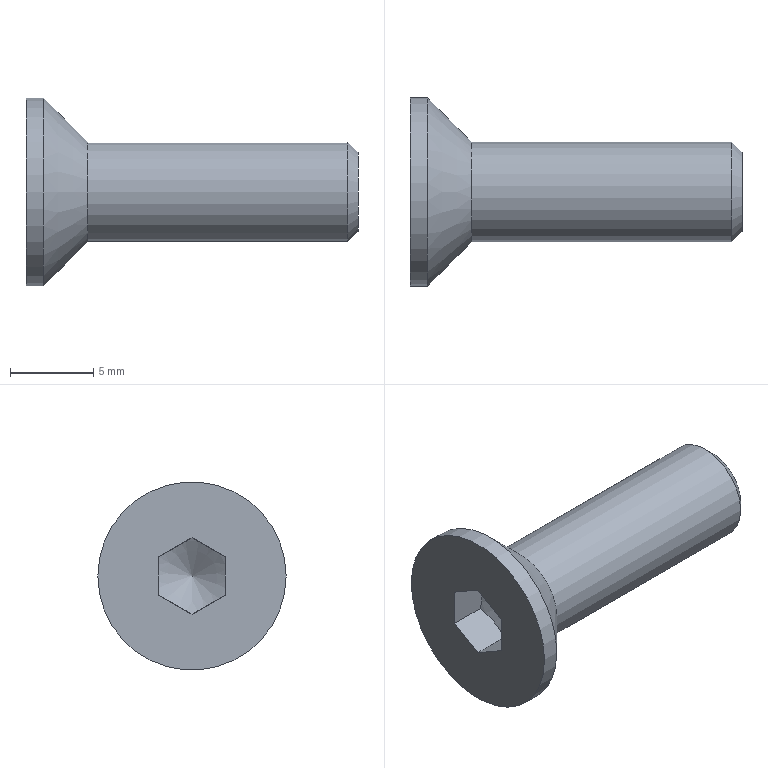Part | STEP file | DIN 7991 - M6  x  20 | 1 solid | 13 faces | box 20 x 11.34 x 11.34 mm | volume 687.937 mm3 | plane 8 | cone 3 | cylinder 2 | commonest cylinder face diameters 6 x1 11.34 x1
STEP:
#1=CARTESIAN_POINT('',(0.,0.,0.));
#2=DIRECTION('',(0.,0.,1.));
#3=DIRECTION('',(1.,0.,0.));
#4=AXIS2_PLACEMENT_3D('',#1,#2,#3);
#5=CARTESIAN_POINT('',(19.387,3.,0.));
#6=VERTEX_POINT('',#5);
#7=CARTESIAN_POINT('',(19.387,0.,0.));
#8=DIRECTION('',(1.,0.,0.));
#9=DIRECTION('',(0.,-1.,0.));
#10=AXIS2_PLACEMENT_3D('',#7,#8,#9);
#11=CIRCLE('',#10,3.);
#12=CARTESIAN_POINT('',(19.693,0.,0.));
#13=DIRECTION('',(-1.,0.,0.));
#14=DIRECTION('',(0.,-1.,0.));
#15=AXIS2_PLACEMENT_3D('',#12,#13,#14);
#16=CONICAL_SURFACE('',#15,2.693,0.7854);
#17=CARTESIAN_POINT('',(12.566,0.3067));
#18=DIRECTION('',(-1.,0.));
#19=VECTOR('',#18,1.);
#20=LINE('',#17,#19);
#21=(GEOMETRIC_REPRESENTATION_CONTEXT(2)PARAMETRIC_REPRESENTATION_CONTEXT()REPRESENTATION_CONTEXT('',''));
#22=DEFINITIONAL_REPRESENTATION('',(#20),#21);
#23=PCURVE('',#16,#22);
#24=CARTESIAN_POINT('',(13.5,0.,0.));
#25=DIRECTION('',(1.,0.,0.));
#26=DIRECTION('',(0.,1.,0.));
#27=AXIS2_PLACEMENT_3D('',#24,#25,#26);
#28=CYLINDRICAL_SURFACE('',#27,3.);
#29=CARTESIAN_POINT('',(-3.142,5.887));
#30=DIRECTION('',(1.,0.));
#31=VECTOR('',#30,1.);
#32=LINE('',#29,#31);
#33=(GEOMETRIC_REPRESENTATION_CONTEXT(2)PARAMETRIC_REPRESENTATION_CONTEXT()REPRESENTATION_CONTEXT('',''));
#34=DEFINITIONAL_REPRESENTATION('',(#32),#33);
#35=PCURVE('',#28,#34);
#36=SURFACE_CURVE('',#11,(#23,#35),.PCURVE_S1.);
#37=EDGE_CURVE('',#6,#6,#36,.T.);
#38=ORIENTED_EDGE('',*,*,#37,.T.);
#39=CARTESIAN_POINT('',(20.,2.387,0.));
#40=VERTEX_POINT('',#39);
#41=CARTESIAN_POINT('',(20.,2.387,0.));
#42=CARTESIAN_POINT('',(19.387,3.,0.));
#43=B_SPLINE_CURVE_WITH_KNOTS('',1,(#41,#42),.UNSPECIFIED.,.F.,.F.,(2,2),(-0.4338,0.4338),.PIECEWISE_BEZIER_KNOTS.);
#44=CARTESIAN_POINT('',(3.142,0.));
#45=DIRECTION('',(0.,1.));
#46=VECTOR('',#45,1.);
#47=LINE('',#44,#46);
#48=(GEOMETRIC_REPRESENTATION_CONTEXT(2)PARAMETRIC_REPRESENTATION_CONTEXT()REPRESENTATION_CONTEXT('',''));
#49=DEFINITIONAL_REPRESENTATION('',(#47),#48);
#50=PCURVE('',#16,#49);
#51=CARTESIAN_POINT('',(9.425,0.));
#52=DIRECTION('',(0.,1.));
#53=VECTOR('',#52,1.);
#54=LINE('',#51,#53);
#55=(GEOMETRIC_REPRESENTATION_CONTEXT(2)PARAMETRIC_REPRESENTATION_CONTEXT()REPRESENTATION_CONTEXT('',''));
#56=DEFINITIONAL_REPRESENTATION('',(#54),#55);
#57=PCURVE('',#16,#56);
#58=SEAM_CURVE('',#43,(#50,#57),.PCURVE_S1.);
#59=EDGE_CURVE('',#40,#6,#58,.T.);
#60=ORIENTED_EDGE('',*,*,#59,.F.);
#61=CARTESIAN_POINT('',(20.,0.,0.));
#62=DIRECTION('',(-1.,0.,0.));
#63=DIRECTION('',(0.,-1.,0.));
#64=AXIS2_PLACEMENT_3D('',#61,#62,#63);
#65=CIRCLE('',#64,2.387);
#66=CARTESIAN_POINT('',(0.,-0.3067));
#67=DIRECTION('',(1.,0.));
#68=VECTOR('',#67,1.);
#69=LINE('',#66,#68);
#70=(GEOMETRIC_REPRESENTATION_CONTEXT(2)PARAMETRIC_REPRESENTATION_CONTEXT()REPRESENTATION_CONTEXT('',''));
#71=DEFINITIONAL_REPRESENTATION('',(#69),#70);
#72=PCURVE('',#16,#71);
#73=CARTESIAN_POINT('',(20.,1.5,0.));
#74=DIRECTION('',(1.,0.,0.));
#75=DIRECTION('',(0.,0.,-1.));
#76=AXIS2_PLACEMENT_3D('',#73,#74,#75);
#77=PLANE('',#76);
#78=CARTESIAN_POINT('',(0.,-3.887));
#79=CARTESIAN_POINT('',(-4.134,-3.887));
#80=CARTESIAN_POINT('',(-2.067,-0.3067));
#81=CARTESIAN_POINT('',(0.,3.273));
#82=CARTESIAN_POINT('',(2.067,-0.3067));
#83=CARTESIAN_POINT('',(4.134,-3.887));
#84=CARTESIAN_POINT('',(0.,-3.887));
#85=(BOUNDED_CURVE()B_SPLINE_CURVE(2,(#78,#79,#80,#81,#82,#83,#84),.UNSPECIFIED.,.T.,.F.)B_SPLINE_CURVE_WITH_KNOTS((1,2,2,2,2,1),(-2.094,0.,2.094,4.189,6.283,8.378),.UNSPECIFIED.)CURVE()GEOMETRIC_REPRESENTATION_ITEM()RATIONAL_B_SPLINE_CURVE((1.,0.5,1.,0.5,1.,0.5,1.))REPRESENTATION_ITEM(''));
#86=(GEOMETRIC_REPRESENTATION_CONTEXT(2)PARAMETRIC_REPRESENTATION_CONTEXT()REPRESENTATION_CONTEXT('',''));
#87=DEFINITIONAL_REPRESENTATION('',(#85),#86);
#88=PCURVE('',#77,#87);
#89=SURFACE_CURVE('',#65,(#72,#88),.PCURVE_S1.);
#90=EDGE_CURVE('',#40,#40,#89,.T.);
#91=ORIENTED_EDGE('',*,*,#90,.T.);
#92=ORIENTED_EDGE('',*,*,#59,.T.);
#93=EDGE_LOOP('',(#38,#60,#91,#92));
#94=FACE_BOUND('',#93,.T.);
#95=ADVANCED_FACE('',(#94),#16,.T.);
#96=CARTESIAN_POINT('',(3.72,3.,0.));
#97=VERTEX_POINT('',#96);
#98=CARTESIAN_POINT('',(3.72,0.,0.));
#99=DIRECTION('',(1.,0.,0.));
#100=DIRECTION('',(0.,1.,0.));
#101=AXIS2_PLACEMENT_3D('',#98,#99,#100);
#102=CIRCLE('',#101,3.);
#103=CARTESIAN_POINT('',(0.,-9.78));
#104=DIRECTION('',(1.,0.));
#105=VECTOR('',#104,1.);
#106=LINE('',#103,#105);
#107=(GEOMETRIC_REPRESENTATION_CONTEXT(2)PARAMETRIC_REPRESENTATION_CONTEXT()REPRESENTATION_CONTEXT('',''));
#108=DEFINITIONAL_REPRESENTATION('',(#106),#107);
#109=PCURVE('',#28,#108);
#110=CARTESIAN_POINT('',(2.385,0.,0.));
#111=DIRECTION('',(-1.,0.,0.));
#112=DIRECTION('',(0.,1.,0.));
#113=AXIS2_PLACEMENT_3D('',#110,#111,#112);
#114=CONICAL_SURFACE('',#113,4.335,0.7854);
#115=CARTESIAN_POINT('',(6.283,-1.335));
#116=DIRECTION('',(-1.,0.));
#117=VECTOR('',#116,1.);
#118=LINE('',#115,#117);
#119=(GEOMETRIC_REPRESENTATION_CONTEXT(2)PARAMETRIC_REPRESENTATION_CONTEXT()REPRESENTATION_CONTEXT('',''));
#120=DEFINITIONAL_REPRESENTATION('',(#118),#119);
#121=PCURVE('',#114,#120);
#122=SURFACE_CURVE('',#102,(#109,#121),.PCURVE_S1.);
#123=EDGE_CURVE('',#97,#97,#122,.T.);
#124=ORIENTED_EDGE('',*,*,#123,.T.);
#125=CARTESIAN_POINT('',(3.72,3.,0.));
#126=CARTESIAN_POINT('',(19.387,3.,0.));
#127=B_SPLINE_CURVE_WITH_KNOTS('',1,(#125,#126),.UNSPECIFIED.,.F.,.F.,(2,2),(-9.78,5.887),.PIECEWISE_BEZIER_KNOTS.);
#128=CARTESIAN_POINT('',(6.283,0.));
#129=DIRECTION('',(0.,1.));
#130=VECTOR('',#129,1.);
#131=LINE('',#128,#130);
#132=(GEOMETRIC_REPRESENTATION_CONTEXT(2)PARAMETRIC_REPRESENTATION_CONTEXT()REPRESENTATION_CONTEXT('',''));
#133=DEFINITIONAL_REPRESENTATION('',(#131),#132);
#134=PCURVE('',#28,#133);
#135=CARTESIAN_POINT('',(0.,0.));
#136=DIRECTION('',(0.,1.));
#137=VECTOR('',#136,1.);
#138=LINE('',#135,#137);
#139=(GEOMETRIC_REPRESENTATION_CONTEXT(2)PARAMETRIC_REPRESENTATION_CONTEXT()REPRESENTATION_CONTEXT('',''));
#140=DEFINITIONAL_REPRESENTATION('',(#138),#139);
#141=PCURVE('',#28,#140);
#142=SEAM_CURVE('',#127,(#134,#141),.PCURVE_S1.);
#143=EDGE_CURVE('',#97,#6,#142,.T.);
#144=ORIENTED_EDGE('',*,*,#143,.T.);
#145=ORIENTED_EDGE('',*,*,#37,.F.);
#146=ORIENTED_EDGE('',*,*,#143,.F.);
#147=EDGE_LOOP('',(#124,#144,#145,#146));
#148=FACE_BOUND('',#147,.T.);
#149=ADVANCED_FACE('',(#148),#28,.T.);
#150=ORIENTED_EDGE('',*,*,#90,.F.);
#151=EDGE_LOOP('',(#150));
#152=FACE_BOUND('',#151,.T.);
#153=ADVANCED_FACE('',(#152),#77,.T.);
#154=CARTESIAN_POINT('',(2.2,-2.,-1.155));
#155=VERTEX_POINT('',#154);
#156=CARTESIAN_POINT('',(2.2,-2.,1.155));
#157=VERTEX_POINT('',#156);
#158=CARTESIAN_POINT('',(2.2,-2.,-1.155));
#159=CARTESIAN_POINT('',(2.533,-2.,0.));
#160=CARTESIAN_POINT('',(2.2,-2.,1.155));
#161=(BOUNDED_CURVE()B_SPLINE_CURVE(2,(#158,#159,#160),.UNSPECIFIED.,.F.,.F.)B_SPLINE_CURVE_WITH_KNOTS((3,3),(0.,0.2337),.PIECEWISE_BEZIER_KNOTS.)CURVE()GEOMETRIC_REPRESENTATION_ITEM()RATIONAL_B_SPLINE_CURVE((1.,1.155,1.))REPRESENTATION_ITEM(''));
#162=CARTESIAN_POINT('',(0.,-2.,-1.155));
#163=DIRECTION('',(0.,-1.,0.));
#164=DIRECTION('',(0.,0.,-1.));
#165=AXIS2_PLACEMENT_3D('',#162,#163,#164);
#166=PLANE('',#165);
#167=CARTESIAN_POINT('',(0.,2.2));
#168=CARTESIAN_POINT('',(-1.155,2.533));
#169=CARTESIAN_POINT('',(-2.309,2.2));
#170=(BOUNDED_CURVE()B_SPLINE_CURVE(2,(#167,#168,#169),.UNSPECIFIED.,.F.,.F.)B_SPLINE_CURVE_WITH_KNOTS((3,3),(0.,0.2337),.PIECEWISE_BEZIER_KNOTS.)CURVE()GEOMETRIC_REPRESENTATION_ITEM()RATIONAL_B_SPLINE_CURVE((1.,1.155,1.))REPRESENTATION_ITEM(''));
#171=(GEOMETRIC_REPRESENTATION_CONTEXT(2)PARAMETRIC_REPRESENTATION_CONTEXT()REPRESENTATION_CONTEXT('',''));
#172=DEFINITIONAL_REPRESENTATION('',(#170),#171);
#173=PCURVE('',#166,#172);
#174=CARTESIAN_POINT('',(2.867,0.,0.));
#175=DIRECTION('',(-1.,0.,0.));
#176=DIRECTION('',(0.,1.,0.));
#177=AXIS2_PLACEMENT_3D('',#174,#175,#176);
#178=CONICAL_SURFACE('',#177,1.155,1.047);
#179=CARTESIAN_POINT('',(8.901,0.6667));
#180=CARTESIAN_POINT('',(8.916,0.655));
#181=CARTESIAN_POINT('',(8.947,0.6331));
#182=CARTESIAN_POINT('',(8.993,0.604));
#183=CARTESIAN_POINT('',(9.04,0.5786));
#184=CARTESIAN_POINT('',(9.087,0.5566));
#185=CARTESIAN_POINT('',(9.134,0.5379));
#186=CARTESIAN_POINT('',(9.182,0.5223));
#187=CARTESIAN_POINT('',(9.23,0.5097));
#188=CARTESIAN_POINT('',(9.279,0.5));
#189=CARTESIAN_POINT('',(9.327,0.4931));
#190=CARTESIAN_POINT('',(9.376,0.4889));
#191=CARTESIAN_POINT('',(9.425,0.4876));
#192=CARTESIAN_POINT('',(9.473,0.4889));
#193=CARTESIAN_POINT('',(9.522,0.4931));
#194=CARTESIAN_POINT('',(9.571,0.5));
#195=CARTESIAN_POINT('',(9.619,0.5097));
#196=CARTESIAN_POINT('',(9.667,0.5223));
#197=CARTESIAN_POINT('',(9.715,0.5379));
#198=CARTESIAN_POINT('',(9.763,0.5566));
#199=CARTESIAN_POINT('',(9.81,0.5786));
#200=CARTESIAN_POINT('',(9.856,0.604));
#201=CARTESIAN_POINT('',(9.903,0.6331));
#202=CARTESIAN_POINT('',(9.933,0.655));
#203=CARTESIAN_POINT('',(9.948,0.6667));
#204=B_SPLINE_CURVE_WITH_KNOTS('',3,(#179,#180,#181,#182,#183,#184,#185,#186,#187,#188,#189,#190,#191,#192,#193,#194,#195,#196,#197,#198,#199,#200,#201,#202,#203),.UNSPECIFIED.,.F.,.F.,(4,1,1,1,1,1,1,1,1,1,1,1,1,1,1,1,1,1,1,1,1,1,4),(0.,0.01062,0.02124,0.03187,0.04249,0.05311,0.06373,0.07436,0.08498,0.0956,0.1062,0.1168,0.1275,0.1381,0.1487,0.1593,0.17,0.1806,0.1912,0.2018,0.2124,0.2231,0.2337),.QUASI_UNIFORM_KNOTS.);
#205=(GEOMETRIC_REPRESENTATION_CONTEXT(2)PARAMETRIC_REPRESENTATION_CONTEXT()REPRESENTATION_CONTEXT('',''));
#206=DEFINITIONAL_REPRESENTATION('',(#204),#205);
#207=PCURVE('',#178,#206);
#208=SURFACE_CURVE('',#161,(#173,#207),.PCURVE_S1.);
#209=EDGE_CURVE('',#155,#157,#208,.T.);
#210=ORIENTED_EDGE('',*,*,#209,.F.);
#211=CARTESIAN_POINT('',(0.,-2.,-1.155));
#212=VERTEX_POINT('',#211);
#213=CARTESIAN_POINT('',(1.1,-2.,-1.155));
#214=DIRECTION('',(-1.,0.,0.));
#215=VECTOR('',#214,1.);
#216=LINE('',#213,#215);
#217=CARTESIAN_POINT('',(0.,1.1));
#218=DIRECTION('',(0.,-1.));
#219=VECTOR('',#218,1.);
#220=LINE('',#217,#219);
#221=(GEOMETRIC_REPRESENTATION_CONTEXT(2)PARAMETRIC_REPRESENTATION_CONTEXT()REPRESENTATION_CONTEXT('',''));
#222=DEFINITIONAL_REPRESENTATION('',(#220),#221);
#223=PCURVE('',#166,#222);
#224=CARTESIAN_POINT('',(0.,0.,-2.309));
#225=DIRECTION('',(0.,-0.5,-0.866));
#226=DIRECTION('',(-1.,0.,0.));
#227=AXIS2_PLACEMENT_3D('',#224,#225,#226);
#228=PLANE('',#227);
#229=CARTESIAN_POINT('',(-1.1,-2.309));
#230=DIRECTION('',(1.,0.));
#231=VECTOR('',#230,1.);
#232=LINE('',#229,#231);
#233=(GEOMETRIC_REPRESENTATION_CONTEXT(2)PARAMETRIC_REPRESENTATION_CONTEXT()REPRESENTATION_CONTEXT('',''));
#234=DEFINITIONAL_REPRESENTATION('',(#232),#233);
#235=PCURVE('',#228,#234);
#236=SURFACE_CURVE('',#216,(#223,#235),.PCURVE_S1.);
#237=EDGE_CURVE('',#155,#212,#236,.T.);
#238=ORIENTED_EDGE('',*,*,#237,.T.);
#239=CARTESIAN_POINT('',(0.,-2.,1.155));
#240=VERTEX_POINT('',#239);
#241=CARTESIAN_POINT('',(0.,-2.,-0.5221));
#242=DIRECTION('',(0.,0.,-1.));
#243=VECTOR('',#242,1.);
#244=LINE('',#241,#243);
#245=CARTESIAN_POINT('',(-0.6326,0.));
#246=DIRECTION('',(1.,0.));
#247=VECTOR('',#246,1.);
#248=LINE('',#245,#247);
#249=(GEOMETRIC_REPRESENTATION_CONTEXT(2)PARAMETRIC_REPRESENTATION_CONTEXT()REPRESENTATION_CONTEXT('',''));
#250=DEFINITIONAL_REPRESENTATION('',(#248),#249);
#251=PCURVE('',#166,#250);
#252=CARTESIAN_POINT('',(0.,3.99,0.));
#253=DIRECTION('',(-1.,0.,0.));
#254=DIRECTION('',(0.,0.,1.));
#255=AXIS2_PLACEMENT_3D('',#252,#253,#254);
#256=PLANE('',#255);
#257=CARTESIAN_POINT('',(-0.5221,-5.99));
#258=DIRECTION('',(-1.,0.));
#259=VECTOR('',#258,1.);
#260=LINE('',#257,#259);
#261=(GEOMETRIC_REPRESENTATION_CONTEXT(2)PARAMETRIC_REPRESENTATION_CONTEXT()REPRESENTATION_CONTEXT('',''));
#262=DEFINITIONAL_REPRESENTATION('',(#260),#261);
#263=PCURVE('',#256,#262);
#264=SURFACE_CURVE('',#244,(#251,#263),.PCURVE_S1.);
#265=EDGE_CURVE('',#240,#212,#264,.T.);
#266=ORIENTED_EDGE('',*,*,#265,.F.);
#267=CARTESIAN_POINT('',(1.1,-2.,1.155));
#268=DIRECTION('',(-1.,0.,0.));
#269=VECTOR('',#268,1.);
#270=LINE('',#267,#269);
#271=CARTESIAN_POINT('',(-2.309,1.1));
#272=DIRECTION('',(0.,-1.));
#273=VECTOR('',#272,1.);
#274=LINE('',#271,#273);
#275=(GEOMETRIC_REPRESENTATION_CONTEXT(2)PARAMETRIC_REPRESENTATION_CONTEXT()REPRESENTATION_CONTEXT('',''));
#276=DEFINITIONAL_REPRESENTATION('',(#274),#275);
#277=PCURVE('',#166,#276);
#278=CARTESIAN_POINT('',(0.,-2.,1.155));
#279=DIRECTION('',(0.,-0.5,0.866));
#280=DIRECTION('',(1.,0.,0.));
#281=AXIS2_PLACEMENT_3D('',#278,#279,#280);
#282=PLANE('',#281);
#283=CARTESIAN_POINT('',(1.1,0.));
#284=DIRECTION('',(-1.,0.));
#285=VECTOR('',#284,1.);
#286=LINE('',#283,#285);
#287=(GEOMETRIC_REPRESENTATION_CONTEXT(2)PARAMETRIC_REPRESENTATION_CONTEXT()REPRESENTATION_CONTEXT('',''));
#288=DEFINITIONAL_REPRESENTATION('',(#286),#287);
#289=PCURVE('',#282,#288);
#290=SURFACE_CURVE('',#270,(#277,#289),.PCURVE_S1.);
#291=EDGE_CURVE('',#157,#240,#290,.T.);
#292=ORIENTED_EDGE('',*,*,#291,.F.);
#293=EDGE_LOOP('',(#210,#238,#266,#292));
#294=FACE_BOUND('',#293,.T.);
#295=ADVANCED_FACE('',(#294),#166,.F.);
#296=CARTESIAN_POINT('',(2.2,0.,-2.309));
#297=VERTEX_POINT('',#296);
#298=CARTESIAN_POINT('',(2.2,0.,-2.309));
#299=CARTESIAN_POINT('',(2.533,-1.,-1.732));
#300=CARTESIAN_POINT('',(2.2,-2.,-1.155));
#301=(BOUNDED_CURVE()B_SPLINE_CURVE(2,(#298,#299,#300),.UNSPECIFIED.,.F.,.F.)B_SPLINE_CURVE_WITH_KNOTS((3,3),(0.,0.2337),.PIECEWISE_BEZIER_KNOTS.)CURVE()GEOMETRIC_REPRESENTATION_ITEM()RATIONAL_B_SPLINE_CURVE((1.,1.155,1.))REPRESENTATION_ITEM(''));
#302=CARTESIAN_POINT('',(-2.2,0.));
#303=CARTESIAN_POINT('',(-2.533,-1.155));
#304=CARTESIAN_POINT('',(-2.2,-2.309));
#305=(BOUNDED_CURVE()B_SPLINE_CURVE(2,(#302,#303,#304),.UNSPECIFIED.,.F.,.F.)B_SPLINE_CURVE_WITH_KNOTS((3,3),(0.,0.2337),.PIECEWISE_BEZIER_KNOTS.)CURVE()GEOMETRIC_REPRESENTATION_ITEM()RATIONAL_B_SPLINE_CURVE((1.,1.155,1.))REPRESENTATION_ITEM(''));
#306=(GEOMETRIC_REPRESENTATION_CONTEXT(2)PARAMETRIC_REPRESENTATION_CONTEXT()REPRESENTATION_CONTEXT('',''));
#307=DEFINITIONAL_REPRESENTATION('',(#305),#306);
#308=PCURVE('',#228,#307);
#309=CARTESIAN_POINT('',(7.854,0.6667));
#310=CARTESIAN_POINT('',(7.869,0.655));
#311=CARTESIAN_POINT('',(7.9,0.6331));
#312=CARTESIAN_POINT('',(7.946,0.604));
#313=CARTESIAN_POINT('',(7.993,0.5786));
#314=CARTESIAN_POINT('',(8.04,0.5566));
#315=CARTESIAN_POINT('',(8.087,0.5379));
#316=CARTESIAN_POINT('',(8.135,0.5223));
#317=CARTESIAN_POINT('',(8.183,0.5097));
#318=CARTESIAN_POINT('',(8.232,0.5));
#319=CARTESIAN_POINT('',(8.28,0.4931));
#320=CARTESIAN_POINT('',(8.329,0.4889));
#321=CARTESIAN_POINT('',(8.378,0.4876));
#322=CARTESIAN_POINT('',(8.426,0.4889));
#323=CARTESIAN_POINT('',(8.475,0.4931));
#324=CARTESIAN_POINT('',(8.524,0.5));
#325=CARTESIAN_POINT('',(8.572,0.5097));
#326=CARTESIAN_POINT('',(8.62,0.5223));
#327=CARTESIAN_POINT('',(8.668,0.5379));
#328=CARTESIAN_POINT('',(8.715,0.5566));
#329=CARTESIAN_POINT('',(8.763,0.5786));
#330=CARTESIAN_POINT('',(8.809,0.604));
#331=CARTESIAN_POINT('',(8.856,0.6331));
#332=CARTESIAN_POINT('',(8.886,0.655));
#333=CARTESIAN_POINT('',(8.901,0.6667));
#334=B_SPLINE_CURVE_WITH_KNOTS('',3,(#309,#310,#311,#312,#313,#314,#315,#316,#317,#318,#319,#320,#321,#322,#323,#324,#325,#326,#327,#328,#329,#330,#331,#332,#333),.UNSPECIFIED.,.F.,.F.,(4,1,1,1,1,1,1,1,1,1,1,1,1,1,1,1,1,1,1,1,1,1,4),(0.,0.01062,0.02124,0.03187,0.04249,0.05311,0.06373,0.07436,0.08498,0.0956,0.1062,0.1168,0.1275,0.1381,0.1487,0.1593,0.17,0.1806,0.1912,0.2018,0.2124,0.2231,0.2337),.QUASI_UNIFORM_KNOTS.);
#335=(GEOMETRIC_REPRESENTATION_CONTEXT(2)PARAMETRIC_REPRESENTATION_CONTEXT()REPRESENTATION_CONTEXT('',''));
#336=DEFINITIONAL_REPRESENTATION('',(#334),#335);
#337=PCURVE('',#178,#336);
#338=SURFACE_CURVE('',#301,(#308,#337),.PCURVE_S1.);
#339=EDGE_CURVE('',#297,#155,#338,.T.);
#340=ORIENTED_EDGE('',*,*,#339,.F.);
#341=CARTESIAN_POINT('',(0.,0.,-2.309));
#342=VERTEX_POINT('',#341);
#343=CARTESIAN_POINT('',(1.1,0.,-2.309));
#344=DIRECTION('',(-1.,0.,0.));
#345=VECTOR('',#344,1.);
#346=LINE('',#343,#345);
#347=CARTESIAN_POINT('',(-1.1,0.));
#348=DIRECTION('',(1.,0.));
#349=VECTOR('',#348,1.);
#350=LINE('',#347,#349);
#351=(GEOMETRIC_REPRESENTATION_CONTEXT(2)PARAMETRIC_REPRESENTATION_CONTEXT()REPRESENTATION_CONTEXT('',''));
#352=DEFINITIONAL_REPRESENTATION('',(#350),#351);
#353=PCURVE('',#228,#352);
#354=CARTESIAN_POINT('',(0.,2.,-1.155));
#355=DIRECTION('',(0.,0.5,-0.866));
#356=DIRECTION('',(-1.,0.,0.));
#357=AXIS2_PLACEMENT_3D('',#354,#355,#356);
#358=PLANE('',#357);
#359=CARTESIAN_POINT('',(-1.1,-2.309));
#360=DIRECTION('',(1.,0.));
#361=VECTOR('',#360,1.);
#362=LINE('',#359,#361);
#363=(GEOMETRIC_REPRESENTATION_CONTEXT(2)PARAMETRIC_REPRESENTATION_CONTEXT()REPRESENTATION_CONTEXT('',''));
#364=DEFINITIONAL_REPRESENTATION('',(#362),#363);
#365=PCURVE('',#358,#364);
#366=SURFACE_CURVE('',#346,(#353,#365),.PCURVE_S1.);
#367=EDGE_CURVE('',#297,#342,#366,.T.);
#368=ORIENTED_EDGE('',*,*,#367,.T.);
#369=CARTESIAN_POINT('',(0.,-0.4825,-2.031));
#370=DIRECTION('',(0.,0.866,-0.5));
#371=VECTOR('',#370,1.);
#372=LINE('',#369,#371);
#373=CARTESIAN_POINT('',(0.,-0.5571));
#374=DIRECTION('',(0.,1.));
#375=VECTOR('',#374,1.);
#376=LINE('',#373,#375);
#377=(GEOMETRIC_REPRESENTATION_CONTEXT(2)PARAMETRIC_REPRESENTATION_CONTEXT()REPRESENTATION_CONTEXT('',''));
#378=DEFINITIONAL_REPRESENTATION('',(#376),#377);
#379=PCURVE('',#228,#378);
#380=CARTESIAN_POINT('',(-2.031,-4.472));
#381=DIRECTION('',(-0.5,0.866));
#382=VECTOR('',#381,1.);
#383=LINE('',#380,#382);
#384=(GEOMETRIC_REPRESENTATION_CONTEXT(2)PARAMETRIC_REPRESENTATION_CONTEXT()REPRESENTATION_CONTEXT('',''));
#385=DEFINITIONAL_REPRESENTATION('',(#383),#384);
#386=PCURVE('',#256,#385);
#387=SURFACE_CURVE('',#372,(#379,#386),.PCURVE_S1.);
#388=EDGE_CURVE('',#212,#342,#387,.T.);
#389=ORIENTED_EDGE('',*,*,#388,.F.);
#390=ORIENTED_EDGE('',*,*,#237,.F.);
#391=EDGE_LOOP('',(#340,#368,#389,#390));
#392=FACE_BOUND('',#391,.T.);
#393=ADVANCED_FACE('',(#392),#228,.F.);
#394=CARTESIAN_POINT('',(2.2,2.,-1.155));
#395=VERTEX_POINT('',#394);
#396=CARTESIAN_POINT('',(2.2,2.,-1.155));
#397=CARTESIAN_POINT('',(2.533,1.,-1.732));
#398=CARTESIAN_POINT('',(2.2,0.,-2.309));
#399=(BOUNDED_CURVE()B_SPLINE_CURVE(2,(#396,#397,#398),.UNSPECIFIED.,.F.,.F.)B_SPLINE_CURVE_WITH_KNOTS((3,3),(0.,0.2337),.PIECEWISE_BEZIER_KNOTS.)CURVE()GEOMETRIC_REPRESENTATION_ITEM()RATIONAL_B_SPLINE_CURVE((1.,1.155,1.))REPRESENTATION_ITEM(''));
#400=CARTESIAN_POINT('',(-2.2,0.));
#401=CARTESIAN_POINT('',(-2.533,-1.155));
#402=CARTESIAN_POINT('',(-2.2,-2.309));
#403=(BOUNDED_CURVE()B_SPLINE_CURVE(2,(#400,#401,#402),.UNSPECIFIED.,.F.,.F.)B_SPLINE_CURVE_WITH_KNOTS((3,3),(0.,0.2337),.PIECEWISE_BEZIER_KNOTS.)CURVE()GEOMETRIC_REPRESENTATION_ITEM()RATIONAL_B_SPLINE_CURVE((1.,1.155,1.))REPRESENTATION_ITEM(''));
#404=(GEOMETRIC_REPRESENTATION_CONTEXT(2)PARAMETRIC_REPRESENTATION_CONTEXT()REPRESENTATION_CONTEXT('',''));
#405=DEFINITIONAL_REPRESENTATION('',(#403),#404);
#406=PCURVE('',#358,#405);
#407=CARTESIAN_POINT('',(6.807,0.6667));
#408=CARTESIAN_POINT('',(6.822,0.655));
#409=CARTESIAN_POINT('',(6.852,0.6331));
#410=CARTESIAN_POINT('',(6.899,0.604));
#411=CARTESIAN_POINT('',(6.945,0.5786));
#412=CARTESIAN_POINT('',(6.993,0.5566));
#413=CARTESIAN_POINT('',(7.04,0.5379));
#414=CARTESIAN_POINT('',(7.088,0.5223));
#415=CARTESIAN_POINT('',(7.136,0.5097));
#416=CARTESIAN_POINT('',(7.184,0.5));
#417=CARTESIAN_POINT('',(7.233,0.4931));
#418=CARTESIAN_POINT('',(7.282,0.4889));
#419=CARTESIAN_POINT('',(7.33,0.4876));
#420=CARTESIAN_POINT('',(7.379,0.4889));
#421=CARTESIAN_POINT('',(7.428,0.4931));
#422=CARTESIAN_POINT('',(7.476,0.5));
#423=CARTESIAN_POINT('',(7.525,0.5097));
#424=CARTESIAN_POINT('',(7.573,0.5223));
#425=CARTESIAN_POINT('',(7.621,0.5379));
#426=CARTESIAN_POINT('',(7.668,0.5566));
#427=CARTESIAN_POINT('',(7.715,0.5786));
#428=CARTESIAN_POINT('',(7.762,0.604));
#429=CARTESIAN_POINT('',(7.808,0.6331));
#430=CARTESIAN_POINT('',(7.839,0.655));
#431=CARTESIAN_POINT('',(7.854,0.6667));
#432=B_SPLINE_CURVE_WITH_KNOTS('',3,(#407,#408,#409,#410,#411,#412,#413,#414,#415,#416,#417,#418,#419,#420,#421,#422,#423,#424,#425,#426,#427,#428,#429,#430,#431),.UNSPECIFIED.,.F.,.F.,(4,1,1,1,1,1,1,1,1,1,1,1,1,1,1,1,1,1,1,1,1,1,4),(0.,0.01062,0.02124,0.03187,0.04249,0.05311,0.06373,0.07436,0.08498,0.0956,0.1062,0.1168,0.1275,0.1381,0.1487,0.1593,0.17,0.1806,0.1912,0.2018,0.2124,0.2231,0.2337),.QUASI_UNIFORM_KNOTS.);
#433=(GEOMETRIC_REPRESENTATION_CONTEXT(2)PARAMETRIC_REPRESENTATION_CONTEXT()REPRESENTATION_CONTEXT('',''));
#434=DEFINITIONAL_REPRESENTATION('',(#432),#433);
#435=PCURVE('',#178,#434);
#436=SURFACE_CURVE('',#399,(#406,#435),.PCURVE_S1.);
#437=EDGE_CURVE('',#395,#297,#436,.T.);
#438=ORIENTED_EDGE('',*,*,#437,.F.);
#439=CARTESIAN_POINT('',(0.,2.,-1.155));
#440=VERTEX_POINT('',#439);
#441=CARTESIAN_POINT('',(1.1,2.,-1.155));
#442=DIRECTION('',(-1.,0.,0.));
#443=VECTOR('',#442,1.);
#444=LINE('',#441,#443);
#445=CARTESIAN_POINT('',(-1.1,0.));
#446=DIRECTION('',(1.,0.));
#447=VECTOR('',#446,1.);
#448=LINE('',#445,#447);
#449=(GEOMETRIC_REPRESENTATION_CONTEXT(2)PARAMETRIC_REPRESENTATION_CONTEXT()REPRESENTATION_CONTEXT('',''));
#450=DEFINITIONAL_REPRESENTATION('',(#448),#449);
#451=PCURVE('',#358,#450);
#452=CARTESIAN_POINT('',(0.,2.,1.155));
#453=DIRECTION('',(0.,1.,0.));
#454=DIRECTION('',(0.,0.,1.));
#455=AXIS2_PLACEMENT_3D('',#452,#453,#454);
#456=PLANE('',#455);
#457=CARTESIAN_POINT('',(-2.309,1.1));
#458=DIRECTION('',(0.,-1.));
#459=VECTOR('',#458,1.);
#460=LINE('',#457,#459);
#461=(GEOMETRIC_REPRESENTATION_CONTEXT(2)PARAMETRIC_REPRESENTATION_CONTEXT()REPRESENTATION_CONTEXT('',''));
#462=DEFINITIONAL_REPRESENTATION('',(#460),#461);
#463=PCURVE('',#456,#462);
#464=SURFACE_CURVE('',#444,(#451,#463),.PCURVE_S1.);
#465=EDGE_CURVE('',#395,#440,#464,.T.);
#466=ORIENTED_EDGE('',*,*,#465,.T.);
#467=CARTESIAN_POINT('',(0.,1.565,-1.406));
#468=DIRECTION('',(0.,0.866,0.5));
#469=VECTOR('',#468,1.);
#470=LINE('',#467,#469);
#471=CARTESIAN_POINT('',(0.,-0.5019));
#472=DIRECTION('',(0.,1.));
#473=VECTOR('',#472,1.);
#474=LINE('',#471,#473);
#475=(GEOMETRIC_REPRESENTATION_CONTEXT(2)PARAMETRIC_REPRESENTATION_CONTEXT()REPRESENTATION_CONTEXT('',''));
#476=DEFINITIONAL_REPRESENTATION('',(#474),#475);
#477=PCURVE('',#358,#476);
#478=CARTESIAN_POINT('',(-1.406,-2.424));
#479=DIRECTION('',(0.5,0.866));
#480=VECTOR('',#479,1.);
#481=LINE('',#478,#480);
#482=(GEOMETRIC_REPRESENTATION_CONTEXT(2)PARAMETRIC_REPRESENTATION_CONTEXT()REPRESENTATION_CONTEXT('',''));
#483=DEFINITIONAL_REPRESENTATION('',(#481),#482);
#484=PCURVE('',#256,#483);
#485=SURFACE_CURVE('',#470,(#477,#484),.PCURVE_S1.);
#486=EDGE_CURVE('',#342,#440,#485,.T.);
#487=ORIENTED_EDGE('',*,*,#486,.F.);
#488=ORIENTED_EDGE('',*,*,#367,.F.);
#489=EDGE_LOOP('',(#438,#466,#487,#488));
#490=FACE_BOUND('',#489,.T.);
#491=ADVANCED_FACE('',(#490),#358,.F.);
#492=CARTESIAN_POINT('',(2.2,2.,1.155));
#493=VERTEX_POINT('',#492);
#494=CARTESIAN_POINT('',(2.2,2.,1.155));
#495=CARTESIAN_POINT('',(2.533,2.,0.));
#496=CARTESIAN_POINT('',(2.2,2.,-1.155));
#497=(BOUNDED_CURVE()B_SPLINE_CURVE(2,(#494,#495,#496),.UNSPECIFIED.,.F.,.F.)B_SPLINE_CURVE_WITH_KNOTS((3,3),(0.,0.2337),.PIECEWISE_BEZIER_KNOTS.)CURVE()GEOMETRIC_REPRESENTATION_ITEM()RATIONAL_B_SPLINE_CURVE((1.,1.155,1.))REPRESENTATION_ITEM(''));
#498=CARTESIAN_POINT('',(0.,2.2));
#499=CARTESIAN_POINT('',(-1.155,2.533));
#500=CARTESIAN_POINT('',(-2.309,2.2));
#501=(BOUNDED_CURVE()B_SPLINE_CURVE(2,(#498,#499,#500),.UNSPECIFIED.,.F.,.F.)B_SPLINE_CURVE_WITH_KNOTS((3,3),(0.,0.2337),.PIECEWISE_BEZIER_KNOTS.)CURVE()GEOMETRIC_REPRESENTATION_ITEM()RATIONAL_B_SPLINE_CURVE((1.,1.155,1.))REPRESENTATION_ITEM(''));
#502=(GEOMETRIC_REPRESENTATION_CONTEXT(2)PARAMETRIC_REPRESENTATION_CONTEXT()REPRESENTATION_CONTEXT('',''));
#503=DEFINITIONAL_REPRESENTATION('',(#501),#502);
#504=PCURVE('',#456,#503);
#505=CARTESIAN_POINT('',(5.76,0.6667));
#506=CARTESIAN_POINT('',(5.775,0.655));
#507=CARTESIAN_POINT('',(5.805,0.6331));
#508=CARTESIAN_POINT('',(5.851,0.604));
#509=CARTESIAN_POINT('',(5.898,0.5786));
#510=CARTESIAN_POINT('',(5.945,0.5566));
#511=CARTESIAN_POINT('',(5.993,0.5379));
#512=CARTESIAN_POINT('',(6.041,0.5223));
#513=CARTESIAN_POINT('',(6.089,0.5097));
#514=CARTESIAN_POINT('',(6.137,0.5));
#515=CARTESIAN_POINT('',(6.186,0.4931));
#516=CARTESIAN_POINT('',(6.234,0.4889));
#517=CARTESIAN_POINT('',(6.283,0.4876));
#518=CARTESIAN_POINT('',(6.332,0.4889));
#519=CARTESIAN_POINT('',(6.381,0.4931));
#520=CARTESIAN_POINT('',(6.429,0.5));
#521=CARTESIAN_POINT('',(6.477,0.5097));
#522=CARTESIAN_POINT('',(6.526,0.5223));
#523=CARTESIAN_POINT('',(6.573,0.5379));
#524=CARTESIAN_POINT('',(6.621,0.5566));
#525=CARTESIAN_POINT('',(6.668,0.5786));
#526=CARTESIAN_POINT('',(6.715,0.604));
#527=CARTESIAN_POINT('',(6.761,0.6331));
#528=CARTESIAN_POINT('',(6.792,0.655));
#529=CARTESIAN_POINT('',(6.807,0.6667));
#530=B_SPLINE_CURVE_WITH_KNOTS('',3,(#505,#506,#507,#508,#509,#510,#511,#512,#513,#514,#515,#516,#517,#518,#519,#520,#521,#522,#523,#524,#525,#526,#527,#528,#529),.UNSPECIFIED.,.F.,.F.,(4,1,1,1,1,1,1,1,1,1,1,1,1,1,1,1,1,1,1,1,1,1,4),(0.,0.01062,0.02124,0.03187,0.04249,0.05311,0.06373,0.07436,0.08498,0.0956,0.1062,0.1168,0.1275,0.1381,0.1487,0.1593,0.17,0.1806,0.1912,0.2018,0.2124,0.2231,0.2337),.QUASI_UNIFORM_KNOTS.);
#531=(GEOMETRIC_REPRESENTATION_CONTEXT(2)PARAMETRIC_REPRESENTATION_CONTEXT()REPRESENTATION_CONTEXT('',''));
#532=DEFINITIONAL_REPRESENTATION('',(#530),#531);
#533=PCURVE('',#178,#532);
#534=SURFACE_CURVE('',#497,(#504,#533),.PCURVE_S1.);
#535=EDGE_CURVE('',#493,#395,#534,.T.);
#536=ORIENTED_EDGE('',*,*,#535,.F.);
#537=CARTESIAN_POINT('',(0.,2.,1.155));
#538=VERTEX_POINT('',#537);
#539=CARTESIAN_POINT('',(1.1,2.,1.155));
#540=DIRECTION('',(1.,0.,0.));
#541=VECTOR('',#540,1.);
#542=LINE('',#539,#541);
#543=CARTESIAN_POINT('',(0.,1.1));
#544=DIRECTION('',(0.,1.));
#545=VECTOR('',#544,1.);
#546=LINE('',#543,#545);
#547=(GEOMETRIC_REPRESENTATION_CONTEXT(2)PARAMETRIC_REPRESENTATION_CONTEXT()REPRESENTATION_CONTEXT('',''));
#548=DEFINITIONAL_REPRESENTATION('',(#546),#547);
#549=PCURVE('',#456,#548);
#550=CARTESIAN_POINT('',(0.,0.,2.309));
#551=DIRECTION('',(0.,0.5,0.866));
#552=DIRECTION('',(1.,0.,0.));
#553=AXIS2_PLACEMENT_3D('',#550,#551,#552);
#554=PLANE('',#553);
#555=CARTESIAN_POINT('',(1.1,2.309));
#556=DIRECTION('',(1.,0.));
#557=VECTOR('',#556,1.);
#558=LINE('',#555,#557);
#559=(GEOMETRIC_REPRESENTATION_CONTEXT(2)PARAMETRIC_REPRESENTATION_CONTEXT()REPRESENTATION_CONTEXT('',''));
#560=DEFINITIONAL_REPRESENTATION('',(#558),#559);
#561=PCURVE('',#554,#560);
#562=SURFACE_CURVE('',#542,(#549,#561),.PCURVE_S1.);
#563=EDGE_CURVE('',#538,#493,#562,.T.);
#564=ORIENTED_EDGE('',*,*,#563,.F.);
#565=CARTESIAN_POINT('',(0.,2.,0.6326));
#566=DIRECTION('',(0.,0.,1.));
#567=VECTOR('',#566,1.);
#568=LINE('',#565,#567);
#569=CARTESIAN_POINT('',(-0.5221,0.));
#570=DIRECTION('',(1.,0.));
#571=VECTOR('',#570,1.);
#572=LINE('',#569,#571);
#573=(GEOMETRIC_REPRESENTATION_CONTEXT(2)PARAMETRIC_REPRESENTATION_CONTEXT()REPRESENTATION_CONTEXT('',''));
#574=DEFINITIONAL_REPRESENTATION('',(#572),#573);
#575=PCURVE('',#456,#574);
#576=CARTESIAN_POINT('',(0.6326,-1.99));
#577=DIRECTION('',(1.,0.));
#578=VECTOR('',#577,1.);
#579=LINE('',#576,#578);
#580=(GEOMETRIC_REPRESENTATION_CONTEXT(2)PARAMETRIC_REPRESENTATION_CONTEXT()REPRESENTATION_CONTEXT('',''));
#581=DEFINITIONAL_REPRESENTATION('',(#579),#580);
#582=PCURVE('',#256,#581);
#583=SURFACE_CURVE('',#568,(#575,#582),.PCURVE_S1.);
#584=EDGE_CURVE('',#440,#538,#583,.T.);
#585=ORIENTED_EDGE('',*,*,#584,.F.);
#586=ORIENTED_EDGE('',*,*,#465,.F.);
#587=EDGE_LOOP('',(#536,#564,#585,#586));
#588=FACE_BOUND('',#587,.T.);
#589=ADVANCED_FACE('',(#588),#456,.F.);
#590=CARTESIAN_POINT('',(2.2,0.,2.309));
#591=VERTEX_POINT('',#590);
#592=CARTESIAN_POINT('',(2.2,-2.,1.155));
#593=CARTESIAN_POINT('',(2.533,-1.,1.732));
#594=CARTESIAN_POINT('',(2.2,0.,2.309));
#595=(BOUNDED_CURVE()B_SPLINE_CURVE(2,(#592,#593,#594),.UNSPECIFIED.,.F.,.F.)B_SPLINE_CURVE_WITH_KNOTS((3,3),(0.,0.2337),.PIECEWISE_BEZIER_KNOTS.)CURVE()GEOMETRIC_REPRESENTATION_ITEM()RATIONAL_B_SPLINE_CURVE((1.,1.155,1.))REPRESENTATION_ITEM(''));
#596=CARTESIAN_POINT('',(2.2,0.));
#597=CARTESIAN_POINT('',(2.533,1.155));
#598=CARTESIAN_POINT('',(2.2,2.309));
#599=(BOUNDED_CURVE()B_SPLINE_CURVE(2,(#596,#597,#598),.UNSPECIFIED.,.F.,.F.)B_SPLINE_CURVE_WITH_KNOTS((3,3),(0.,0.2337),.PIECEWISE_BEZIER_KNOTS.)CURVE()GEOMETRIC_REPRESENTATION_ITEM()RATIONAL_B_SPLINE_CURVE((1.,1.155,1.))REPRESENTATION_ITEM(''));
#600=(GEOMETRIC_REPRESENTATION_CONTEXT(2)PARAMETRIC_REPRESENTATION_CONTEXT()REPRESENTATION_CONTEXT('',''));
#601=DEFINITIONAL_REPRESENTATION('',(#599),#600);
#602=PCURVE('',#282,#601);
#603=CARTESIAN_POINT('',(9.948,0.6667));
#604=CARTESIAN_POINT('',(9.964,0.655));
#605=CARTESIAN_POINT('',(9.994,0.6331));
#606=CARTESIAN_POINT('',(10.04,0.604));
#607=CARTESIAN_POINT('',(10.087,0.5786));
#608=CARTESIAN_POINT('',(10.134,0.5566));
#609=CARTESIAN_POINT('',(10.182,0.5379));
#610=CARTESIAN_POINT('',(10.23,0.5223));
#611=CARTESIAN_POINT('',(10.278,0.5097));
#612=CARTESIAN_POINT('',(10.326,0.5));
#613=CARTESIAN_POINT('',(10.375,0.4931));
#614=CARTESIAN_POINT('',(10.423,0.4889));
#615=CARTESIAN_POINT('',(10.472,0.4876));
#616=CARTESIAN_POINT('',(10.521,0.4889));
#617=CARTESIAN_POINT('',(10.569,0.4931));
#618=CARTESIAN_POINT('',(10.618,0.5));
#619=CARTESIAN_POINT('',(10.666,0.5097));
#620=CARTESIAN_POINT('',(10.714,0.5223));
#621=CARTESIAN_POINT('',(10.762,0.5379));
#622=CARTESIAN_POINT('',(10.81,0.5566));
#623=CARTESIAN_POINT('',(10.857,0.5786));
#624=CARTESIAN_POINT('',(10.904,0.604));
#625=CARTESIAN_POINT('',(10.95,0.6331));
#626=CARTESIAN_POINT('',(10.98,0.655));
#627=CARTESIAN_POINT('',(10.996,0.6667));
#628=B_SPLINE_CURVE_WITH_KNOTS('',3,(#603,#604,#605,#606,#607,#608,#609,#610,#611,#612,#613,#614,#615,#616,#617,#618,#619,#620,#621,#622,#623,#624,#625,#626,#627),.UNSPECIFIED.,.F.,.F.,(4,1,1,1,1,1,1,1,1,1,1,1,1,1,1,1,1,1,1,1,1,1,4),(0.,0.01062,0.02124,0.03187,0.04249,0.05311,0.06373,0.07436,0.08498,0.0956,0.1062,0.1168,0.1275,0.1381,0.1487,0.1593,0.17,0.1806,0.1912,0.2018,0.2124,0.2231,0.2337),.QUASI_UNIFORM_KNOTS.);
#629=(GEOMETRIC_REPRESENTATION_CONTEXT(2)PARAMETRIC_REPRESENTATION_CONTEXT()REPRESENTATION_CONTEXT('',''));
#630=DEFINITIONAL_REPRESENTATION('',(#628),#629);
#631=PCURVE('',#178,#630);
#632=SURFACE_CURVE('',#595,(#602,#631),.PCURVE_S1.);
#633=EDGE_CURVE('',#157,#591,#632,.T.);
#634=ORIENTED_EDGE('',*,*,#633,.F.);
#635=ORIENTED_EDGE('',*,*,#291,.T.);
#636=CARTESIAN_POINT('',(0.,0.,2.309));
#637=VERTEX_POINT('',#636);
#638=CARTESIAN_POINT('',(0.,-1.435,1.481));
#639=DIRECTION('',(0.,-0.866,-0.5));
#640=VECTOR('',#639,1.);
#641=LINE('',#638,#640);
#642=CARTESIAN_POINT('',(0.,0.6528));
#643=DIRECTION('',(0.,-1.));
#644=VECTOR('',#643,1.);
#645=LINE('',#642,#644);
#646=(GEOMETRIC_REPRESENTATION_CONTEXT(2)PARAMETRIC_REPRESENTATION_CONTEXT()REPRESENTATION_CONTEXT('',''));
#647=DEFINITIONAL_REPRESENTATION('',(#645),#646);
#648=PCURVE('',#282,#647);
#649=CARTESIAN_POINT('',(1.481,-5.424));
#650=DIRECTION('',(-0.5,-0.866));
#651=VECTOR('',#650,1.);
#652=LINE('',#649,#651);
#653=(GEOMETRIC_REPRESENTATION_CONTEXT(2)PARAMETRIC_REPRESENTATION_CONTEXT()REPRESENTATION_CONTEXT('',''));
#654=DEFINITIONAL_REPRESENTATION('',(#652),#653);
#655=PCURVE('',#256,#654);
#656=SURFACE_CURVE('',#641,(#648,#655),.PCURVE_S1.);
#657=EDGE_CURVE('',#637,#240,#656,.T.);
#658=ORIENTED_EDGE('',*,*,#657,.F.);
#659=CARTESIAN_POINT('',(1.1,0.,2.309));
#660=DIRECTION('',(-1.,0.,0.));
#661=VECTOR('',#660,1.);
#662=LINE('',#659,#661);
#663=CARTESIAN_POINT('',(1.1,2.309));
#664=DIRECTION('',(-1.,0.));
#665=VECTOR('',#664,1.);
#666=LINE('',#663,#665);
#667=(GEOMETRIC_REPRESENTATION_CONTEXT(2)PARAMETRIC_REPRESENTATION_CONTEXT()REPRESENTATION_CONTEXT('',''));
#668=DEFINITIONAL_REPRESENTATION('',(#666),#667);
#669=PCURVE('',#282,#668);
#670=CARTESIAN_POINT('',(1.1,0.));
#671=DIRECTION('',(-1.,0.));
#672=VECTOR('',#671,1.);
#673=LINE('',#670,#672);
#674=(GEOMETRIC_REPRESENTATION_CONTEXT(2)PARAMETRIC_REPRESENTATION_CONTEXT()REPRESENTATION_CONTEXT('',''));
#675=DEFINITIONAL_REPRESENTATION('',(#673),#674);
#676=PCURVE('',#554,#675);
#677=SURFACE_CURVE('',#662,(#669,#676),.PCURVE_S1.);
#678=EDGE_CURVE('',#591,#637,#677,.T.);
#679=ORIENTED_EDGE('',*,*,#678,.F.);
#680=EDGE_LOOP('',(#634,#635,#658,#679));
#681=FACE_BOUND('',#680,.T.);
#682=ADVANCED_FACE('',(#681),#282,.F.);
#683=CARTESIAN_POINT('',(2.2,0.,2.309));
#684=CARTESIAN_POINT('',(2.533,1.,1.732));
#685=CARTESIAN_POINT('',(2.2,2.,1.155));
#686=(BOUNDED_CURVE()B_SPLINE_CURVE(2,(#683,#684,#685),.UNSPECIFIED.,.F.,.F.)B_SPLINE_CURVE_WITH_KNOTS((3,3),(0.,0.2337),.PIECEWISE_BEZIER_KNOTS.)CURVE()GEOMETRIC_REPRESENTATION_ITEM()RATIONAL_B_SPLINE_CURVE((1.,1.155,1.))REPRESENTATION_ITEM(''));
#687=CARTESIAN_POINT('',(2.2,0.));
#688=CARTESIAN_POINT('',(2.533,1.155));
#689=CARTESIAN_POINT('',(2.2,2.309));
#690=(BOUNDED_CURVE()B_SPLINE_CURVE(2,(#687,#688,#689),.UNSPECIFIED.,.F.,.F.)B_SPLINE_CURVE_WITH_KNOTS((3,3),(0.,0.2337),.PIECEWISE_BEZIER_KNOTS.)CURVE()GEOMETRIC_REPRESENTATION_ITEM()RATIONAL_B_SPLINE_CURVE((1.,1.155,1.))REPRESENTATION_ITEM(''));
#691=(GEOMETRIC_REPRESENTATION_CONTEXT(2)PARAMETRIC_REPRESENTATION_CONTEXT()REPRESENTATION_CONTEXT('',''));
#692=DEFINITIONAL_REPRESENTATION('',(#690),#691);
#693=PCURVE('',#554,#692);
#694=CARTESIAN_POINT('',(10.996,0.6667));
#695=CARTESIAN_POINT('',(11.011,0.655));
#696=CARTESIAN_POINT('',(11.041,0.6331));
#697=CARTESIAN_POINT('',(11.087,0.604));
#698=CARTESIAN_POINT('',(11.134,0.5786));
#699=CARTESIAN_POINT('',(11.181,0.5566));
#700=CARTESIAN_POINT('',(11.229,0.5379));
#701=CARTESIAN_POINT('',(11.277,0.5223));
#702=CARTESIAN_POINT('',(11.325,0.5097));
#703=CARTESIAN_POINT('',(11.373,0.5));
#704=CARTESIAN_POINT('',(11.422,0.4931));
#705=CARTESIAN_POINT('',(11.47,0.4889));
#706=CARTESIAN_POINT('',(11.519,0.4876));
#707=CARTESIAN_POINT('',(11.568,0.4889));
#708=CARTESIAN_POINT('',(11.617,0.4931));
#709=CARTESIAN_POINT('',(11.665,0.5));
#710=CARTESIAN_POINT('',(11.713,0.5097));
#711=CARTESIAN_POINT('',(11.762,0.5223));
#712=CARTESIAN_POINT('',(11.809,0.5379));
#713=CARTESIAN_POINT('',(11.857,0.5566));
#714=CARTESIAN_POINT('',(11.904,0.5786));
#715=CARTESIAN_POINT('',(11.951,0.604));
#716=CARTESIAN_POINT('',(11.997,0.6331));
#717=CARTESIAN_POINT('',(12.028,0.655));
#718=CARTESIAN_POINT('',(12.043,0.6667));
#719=B_SPLINE_CURVE_WITH_KNOTS('',3,(#694,#695,#696,#697,#698,#699,#700,#701,#702,#703,#704,#705,#706,#707,#708,#709,#710,#711,#712,#713,#714,#715,#716,#717,#718),.UNSPECIFIED.,.F.,.F.,(4,1,1,1,1,1,1,1,1,1,1,1,1,1,1,1,1,1,1,1,1,1,4),(0.,0.01062,0.02124,0.03187,0.04249,0.05311,0.06373,0.07436,0.08498,0.0956,0.1062,0.1168,0.1275,0.1381,0.1487,0.1593,0.17,0.1806,0.1912,0.2018,0.2124,0.2231,0.2337),.QUASI_UNIFORM_KNOTS.);
#720=(GEOMETRIC_REPRESENTATION_CONTEXT(2)PARAMETRIC_REPRESENTATION_CONTEXT()REPRESENTATION_CONTEXT('',''));
#721=DEFINITIONAL_REPRESENTATION('',(#719),#720);
#722=PCURVE('',#178,#721);
#723=SURFACE_CURVE('',#686,(#693,#722),.PCURVE_S1.);
#724=EDGE_CURVE('',#591,#493,#723,.T.);
#725=ORIENTED_EDGE('',*,*,#724,.F.);
#726=ORIENTED_EDGE('',*,*,#678,.T.);
#727=CARTESIAN_POINT('',(0.,0.5175,2.011));
#728=DIRECTION('',(0.,-0.866,0.5));
#729=VECTOR('',#728,1.);
#730=LINE('',#727,#729);
#731=CARTESIAN_POINT('',(0.,0.5976));
#732=DIRECTION('',(0.,-1.));
#733=VECTOR('',#732,1.);
#734=LINE('',#731,#733);
#735=(GEOMETRIC_REPRESENTATION_CONTEXT(2)PARAMETRIC_REPRESENTATION_CONTEXT()REPRESENTATION_CONTEXT('',''));
#736=DEFINITIONAL_REPRESENTATION('',(#734),#735);
#737=PCURVE('',#554,#736);
#738=CARTESIAN_POINT('',(2.011,-3.472));
#739=DIRECTION('',(0.5,-0.866));
#740=VECTOR('',#739,1.);
#741=LINE('',#738,#740);
#742=(GEOMETRIC_REPRESENTATION_CONTEXT(2)PARAMETRIC_REPRESENTATION_CONTEXT()REPRESENTATION_CONTEXT('',''));
#743=DEFINITIONAL_REPRESENTATION('',(#741),#742);
#744=PCURVE('',#256,#743);
#745=SURFACE_CURVE('',#730,(#737,#744),.PCURVE_S1.);
#746=EDGE_CURVE('',#538,#637,#745,.T.);
#747=ORIENTED_EDGE('',*,*,#746,.F.);
#748=ORIENTED_EDGE('',*,*,#563,.T.);
#749=EDGE_LOOP('',(#725,#726,#747,#748));
#750=FACE_BOUND('',#749,.T.);
#751=ADVANCED_FACE('',(#750),#554,.F.);
#752=ORIENTED_EDGE('',*,*,#724,.F.);
#753=ORIENTED_EDGE('',*,*,#633,.F.);
#754=ORIENTED_EDGE('',*,*,#209,.F.);
#755=ORIENTED_EDGE('',*,*,#339,.F.);
#756=ORIENTED_EDGE('',*,*,#437,.F.);
#757=ORIENTED_EDGE('',*,*,#535,.F.);
#758=CARTESIAN_POINT('',(3.533,0.,0.));
#759=VERTEX_POINT('',#758);
#760=CARTESIAN_POINT('',(3.533,0.,0.));
#761=CARTESIAN_POINT('',(2.2,2.,1.155));
#762=B_SPLINE_CURVE_WITH_KNOTS('',1,(#760,#761),.UNSPECIFIED.,.F.,.F.,(2,2),(-1.333,1.333),.PIECEWISE_BEZIER_KNOTS.);
#763=CARTESIAN_POINT('',(5.76,0.));
#764=DIRECTION('',(0.,1.));
#765=VECTOR('',#764,1.);
#766=LINE('',#763,#765);
#767=(GEOMETRIC_REPRESENTATION_CONTEXT(2)PARAMETRIC_REPRESENTATION_CONTEXT()REPRESENTATION_CONTEXT('',''));
#768=DEFINITIONAL_REPRESENTATION('',(#766),#767);
#769=PCURVE('',#178,#768);
#770=CARTESIAN_POINT('',(12.043,0.));
#771=DIRECTION('',(0.,1.));
#772=VECTOR('',#771,1.);
#773=LINE('',#770,#772);
#774=(GEOMETRIC_REPRESENTATION_CONTEXT(2)PARAMETRIC_REPRESENTATION_CONTEXT()REPRESENTATION_CONTEXT('',''));
#775=DEFINITIONAL_REPRESENTATION('',(#773),#774);
#776=PCURVE('',#178,#775);
#777=SEAM_CURVE('',#762,(#769,#776),.PCURVE_S1.);
#778=EDGE_CURVE('',#759,#493,#777,.T.);
#779=ORIENTED_EDGE('',*,*,#778,.F.);
#780=ORIENTED_EDGE('',*,*,#778,.T.);
#781=EDGE_LOOP('',(#752,#753,#754,#755,#756,#757,#779,#780));
#782=FACE_BOUND('',#781,.F.);
#783=ADVANCED_FACE('',(#782),#178,.F.);
#784=CARTESIAN_POINT('',(0.,5.67,0.));
#785=VERTEX_POINT('',#784);
#786=CARTESIAN_POINT('',(0.,0.,0.));
#787=DIRECTION('',(1.,0.,0.));
#788=DIRECTION('',(0.,1.,0.));
#789=AXIS2_PLACEMENT_3D('',#786,#787,#788);
#790=CIRCLE('',#789,5.67);
#791=CARTESIAN_POINT('',(0.,1.68));
#792=CARTESIAN_POINT('',(9.821,1.68));
#793=CARTESIAN_POINT('',(4.91,-6.825));
#794=CARTESIAN_POINT('',(0.,-15.33));
#795=CARTESIAN_POINT('',(-4.91,-6.825));
#796=CARTESIAN_POINT('',(-9.821,1.68));
#797=CARTESIAN_POINT('',(0.,1.68));
#798=(BOUNDED_CURVE()B_SPLINE_CURVE(2,(#791,#792,#793,#794,#795,#796,#797),.UNSPECIFIED.,.T.,.F.)B_SPLINE_CURVE_WITH_KNOTS((1,2,2,2,2,1),(-2.094,0.,2.094,4.189,6.283,8.378),.UNSPECIFIED.)CURVE()GEOMETRIC_REPRESENTATION_ITEM()RATIONAL_B_SPLINE_CURVE((1.,0.5,1.,0.5,1.,0.5,1.))REPRESENTATION_ITEM(''));
#799=(GEOMETRIC_REPRESENTATION_CONTEXT(2)PARAMETRIC_REPRESENTATION_CONTEXT()REPRESENTATION_CONTEXT('',''));
#800=DEFINITIONAL_REPRESENTATION('',(#798),#799);
#801=PCURVE('',#256,#800);
#802=CARTESIAN_POINT('',(0.525,0.,0.));
#803=DIRECTION('',(1.,0.,0.));
#804=DIRECTION('',(0.,1.,0.));
#805=AXIS2_PLACEMENT_3D('',#802,#803,#804);
#806=CYLINDRICAL_SURFACE('',#805,5.67);
#807=CARTESIAN_POINT('',(0.,-0.525));
#808=DIRECTION('',(1.,0.));
#809=VECTOR('',#808,1.);
#810=LINE('',#807,#809);
#811=(GEOMETRIC_REPRESENTATION_CONTEXT(2)PARAMETRIC_REPRESENTATION_CONTEXT()REPRESENTATION_CONTEXT('',''));
#812=DEFINITIONAL_REPRESENTATION('',(#810),#811);
#813=PCURVE('',#806,#812);
#814=SURFACE_CURVE('',#790,(#801,#813),.PCURVE_S1.);
#815=EDGE_CURVE('',#785,#785,#814,.T.);
#816=ORIENTED_EDGE('',*,*,#815,.F.);
#817=EDGE_LOOP('',(#816));
#818=FACE_BOUND('',#817,.T.);
#819=ORIENTED_EDGE('',*,*,#584,.T.);
#820=ORIENTED_EDGE('',*,*,#746,.T.);
#821=ORIENTED_EDGE('',*,*,#657,.T.);
#822=ORIENTED_EDGE('',*,*,#265,.T.);
#823=ORIENTED_EDGE('',*,*,#388,.T.);
#824=ORIENTED_EDGE('',*,*,#486,.T.);
#825=EDGE_LOOP('',(#819,#820,#821,#822,#823,#824));
#826=FACE_BOUND('',#825,.T.);
#827=ADVANCED_FACE('',(#818,#826),#256,.T.);
#828=CARTESIAN_POINT('',(1.05,5.67,0.));
#829=VERTEX_POINT('',#828);
#830=CARTESIAN_POINT('',(1.05,0.,0.));
#831=DIRECTION('',(1.,0.,0.));
#832=DIRECTION('',(0.,1.,0.));
#833=AXIS2_PLACEMENT_3D('',#830,#831,#832);
#834=CIRCLE('',#833,5.67);
#835=CARTESIAN_POINT('',(0.,0.525));
#836=DIRECTION('',(1.,0.));
#837=VECTOR('',#836,1.);
#838=LINE('',#835,#837);
#839=(GEOMETRIC_REPRESENTATION_CONTEXT(2)PARAMETRIC_REPRESENTATION_CONTEXT()REPRESENTATION_CONTEXT('',''));
#840=DEFINITIONAL_REPRESENTATION('',(#838),#839);
#841=PCURVE('',#806,#840);
#842=CARTESIAN_POINT('',(6.283,1.335));
#843=DIRECTION('',(-1.,0.));
#844=VECTOR('',#843,1.);
#845=LINE('',#842,#844);
#846=(GEOMETRIC_REPRESENTATION_CONTEXT(2)PARAMETRIC_REPRESENTATION_CONTEXT()REPRESENTATION_CONTEXT('',''));
#847=DEFINITIONAL_REPRESENTATION('',(#845),#846);
#848=PCURVE('',#114,#847);
#849=SURFACE_CURVE('',#834,(#841,#848),.PCURVE_S1.);
#850=EDGE_CURVE('',#829,#829,#849,.T.);
#851=ORIENTED_EDGE('',*,*,#850,.F.);
#852=CARTESIAN_POINT('',(0.,5.67,0.));
#853=CARTESIAN_POINT('',(1.05,5.67,0.));
#854=B_SPLINE_CURVE_WITH_KNOTS('',1,(#852,#853),.UNSPECIFIED.,.F.,.F.,(2,2),(-0.525,0.525),.PIECEWISE_BEZIER_KNOTS.);
#855=CARTESIAN_POINT('',(0.,0.));
#856=DIRECTION('',(0.,1.));
#857=VECTOR('',#856,1.);
#858=LINE('',#855,#857);
#859=(GEOMETRIC_REPRESENTATION_CONTEXT(2)PARAMETRIC_REPRESENTATION_CONTEXT()REPRESENTATION_CONTEXT('',''));
#860=DEFINITIONAL_REPRESENTATION('',(#858),#859);
#861=PCURVE('',#806,#860);
#862=CARTESIAN_POINT('',(6.283,0.));
#863=DIRECTION('',(0.,1.));
#864=VECTOR('',#863,1.);
#865=LINE('',#862,#864);
#866=(GEOMETRIC_REPRESENTATION_CONTEXT(2)PARAMETRIC_REPRESENTATION_CONTEXT()REPRESENTATION_CONTEXT('',''));
#867=DEFINITIONAL_REPRESENTATION('',(#865),#866);
#868=PCURVE('',#806,#867);
#869=SEAM_CURVE('',#854,(#861,#868),.PCURVE_S1.);
#870=EDGE_CURVE('',#785,#829,#869,.T.);
#871=ORIENTED_EDGE('',*,*,#870,.F.);
#872=ORIENTED_EDGE('',*,*,#815,.T.);
#873=ORIENTED_EDGE('',*,*,#870,.T.);
#874=EDGE_LOOP('',(#851,#871,#872,#873));
#875=FACE_BOUND('',#874,.T.);
#876=ADVANCED_FACE('',(#875),#806,.T.);
#877=ORIENTED_EDGE('',*,*,#123,.F.);
#878=CARTESIAN_POINT('',(3.72,3.,0.));
#879=CARTESIAN_POINT('',(1.05,5.67,0.));
#880=B_SPLINE_CURVE_WITH_KNOTS('',1,(#878,#879),.UNSPECIFIED.,.F.,.F.,(2,2),(-1.888,1.888),.PIECEWISE_BEZIER_KNOTS.);
#881=CARTESIAN_POINT('',(6.283,0.));
#882=DIRECTION('',(0.,1.));
#883=VECTOR('',#882,1.);
#884=LINE('',#881,#883);
#885=(GEOMETRIC_REPRESENTATION_CONTEXT(2)PARAMETRIC_REPRESENTATION_CONTEXT()REPRESENTATION_CONTEXT('',''));
#886=DEFINITIONAL_REPRESENTATION('',(#884),#885);
#887=PCURVE('',#114,#886);
#888=CARTESIAN_POINT('',(0.,0.));
#889=DIRECTION('',(0.,1.));
#890=VECTOR('',#889,1.);
#891=LINE('',#888,#890);
#892=(GEOMETRIC_REPRESENTATION_CONTEXT(2)PARAMETRIC_REPRESENTATION_CONTEXT()REPRESENTATION_CONTEXT('',''));
#893=DEFINITIONAL_REPRESENTATION('',(#891),#892);
#894=PCURVE('',#114,#893);
#895=SEAM_CURVE('',#880,(#887,#894),.PCURVE_S1.);
#896=EDGE_CURVE('',#97,#829,#895,.T.);
#897=ORIENTED_EDGE('',*,*,#896,.T.);
#898=ORIENTED_EDGE('',*,*,#850,.T.);
#899=ORIENTED_EDGE('',*,*,#896,.F.);
#900=EDGE_LOOP('',(#877,#897,#898,#899));
#901=FACE_BOUND('',#900,.T.);
#902=ADVANCED_FACE('',(#901),#114,.T.);
#903=CLOSED_SHELL('',(#95,#149,#153,#295,#393,#491,#589,#682,#751,#783,#827,#876,#902));
#904=MANIFOLD_SOLID_BREP('',#903);
#905=(LENGTH_UNIT()NAMED_UNIT(*)SI_UNIT(.MILLI.,.METRE.));
#906=UNCERTAINTY_MEASURE_WITH_UNIT(LENGTH_MEASURE(0.000002),#905,'','');
#907=(NAMED_UNIT(*)PLANE_ANGLE_UNIT()SI_UNIT($,.RADIAN.));
#908=(NAMED_UNIT(*)SI_UNIT($,.STERADIAN.)SOLID_ANGLE_UNIT());
#909=(GEOMETRIC_REPRESENTATION_CONTEXT(3)GLOBAL_UNCERTAINTY_ASSIGNED_CONTEXT((#906))GLOBAL_UNIT_ASSIGNED_CONTEXT((#905,#907,#908))REPRESENTATION_CONTEXT('',''));
#910=ADVANCED_BREP_SHAPE_REPRESENTATION('',(#4,#904),#909);